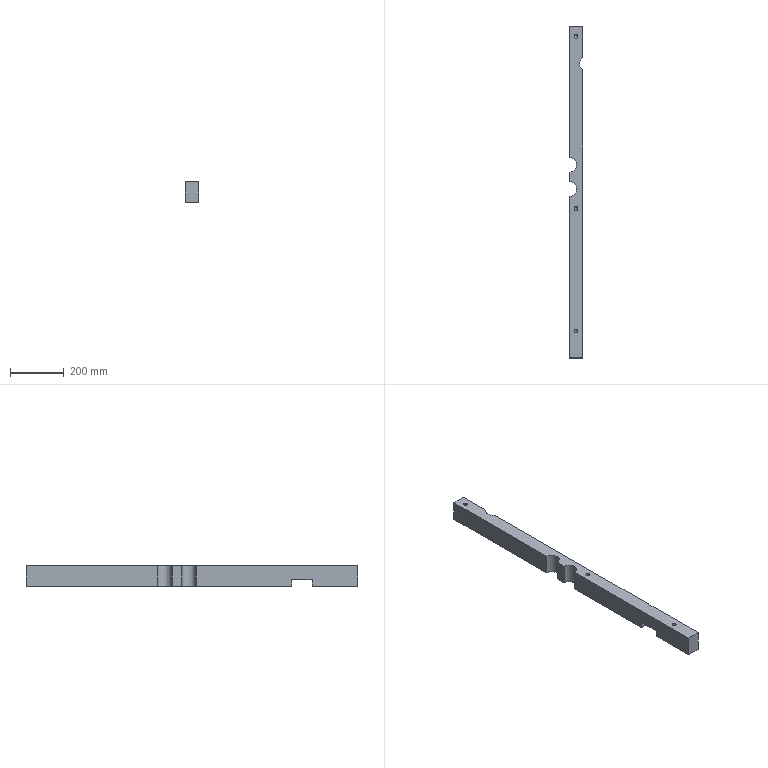Part | NX | features 3 2 | 1 solid | 30 faces | box 50 x 1233 x 75.5 mm | volume 4350206 mm3 | plane 14 | cylinder 10 | cone 6 | commonest cylinder face diameters 14.1 x6 54 x4
STEP:
#1=CARTESIAN_POINT('',(1337.05,-117.5,256.5));
#2=VERTEX_POINT('',#1);
#3=CARTESIAN_POINT('',(1330.,-117.5,256.5));
#4=DIRECTION('',(0.,0.,-1.));
#5=DIRECTION('',(1.,0.,0.));
#6=AXIS2_PLACEMENT_3D('',#3,#4,#5);
#7=CIRCLE('',#6,7.05);
#8=EDGE_CURVE('',#2,#2,#7,.T.);
#9=ORIENTED_EDGE('',*,*,#8,.T.);
#10=EDGE_LOOP('',(#9));
#11=FACE_BOUND('',#10,.T.);
#12=CARTESIAN_POINT('',(1305.,-672.5,256.5));
#13=VERTEX_POINT('',#12);
#14=CARTESIAN_POINT('',(1305.,-72.,256.5));
#15=VERTEX_POINT('',#14);
#16=CARTESIAN_POINT('',(1305.,193.,256.5));
#17=DIRECTION('',(0.,1.,0.));
#18=VECTOR('',#17,1000.);
#19=LINE('',#16,#18);
#20=EDGE_CURVE('',#13,#15,#19,.T.);
#21=ORIENTED_EDGE('',*,*,#20,.F.);
#22=CARTESIAN_POINT('',(1355.,-672.5,256.5));
#23=VERTEX_POINT('',#22);
#24=CARTESIAN_POINT('',(1210.,-672.5,256.5));
#25=DIRECTION('',(-1.,0.,0.));
#26=VECTOR('',#25,1000.);
#27=LINE('',#24,#26);
#28=EDGE_CURVE('',#23,#13,#27,.T.);
#29=ORIENTED_EDGE('',*,*,#28,.F.);
#30=CARTESIAN_POINT('',(1355.,-430.198,256.5));
#31=VERTEX_POINT('',#30);
#32=CARTESIAN_POINT('',(1355.,-526.,256.5));
#33=DIRECTION('',(0.,1.,0.));
#34=VECTOR('',#33,1000.);
#35=LINE('',#32,#34);
#36=EDGE_CURVE('',#23,#31,#35,.T.);
#37=ORIENTED_EDGE('',*,*,#36,.T.);
#38=CARTESIAN_POINT('',(1355.,-409.802,256.5));
#39=VERTEX_POINT('',#38);
#40=CARTESIAN_POINT('',(1380.,-420.,256.5));
#41=DIRECTION('',(0.,0.,1.));
#42=DIRECTION('',(1.,0.,0.));
#43=AXIS2_PLACEMENT_3D('',#40,#41,#42);
#44=CIRCLE('',#43,27.);
#45=EDGE_CURVE('',#39,#31,#44,.T.);
#46=ORIENTED_EDGE('',*,*,#45,.F.);
#47=CARTESIAN_POINT('',(1355.,397.55,256.5));
#48=VERTEX_POINT('',#47);
#49=CARTESIAN_POINT('',(1355.,193.,256.5));
#50=DIRECTION('',(0.,-1.,0.));
#51=VECTOR('',#50,1000.);
#52=LINE('',#49,#51);
#53=EDGE_CURVE('',#48,#39,#52,.T.);
#54=ORIENTED_EDGE('',*,*,#53,.F.);
#55=CARTESIAN_POINT('',(1355.,442.45,256.5));
#56=VERTEX_POINT('',#55);
#57=CARTESIAN_POINT('',(1370.,420.,256.5));
#58=DIRECTION('',(0.,0.,-1.));
#59=DIRECTION('',(1.,0.,0.));
#60=AXIS2_PLACEMENT_3D('',#57,#58,#59);
#61=CIRCLE('',#60,27.);
#62=EDGE_CURVE('',#48,#56,#61,.T.);
#63=ORIENTED_EDGE('',*,*,#62,.T.);
#64=CARTESIAN_POINT('',(1355.,560.5,256.5));
#65=VERTEX_POINT('',#64);
#66=CARTESIAN_POINT('',(1355.,193.,256.5));
#67=DIRECTION('',(0.,-1.,0.));
#68=VECTOR('',#67,1000.);
#69=LINE('',#66,#68);
#70=EDGE_CURVE('',#65,#56,#69,.T.);
#71=ORIENTED_EDGE('',*,*,#70,.F.);
#72=CARTESIAN_POINT('',(1305.,560.5,256.5));
#73=VERTEX_POINT('',#72);
#74=CARTESIAN_POINT('',(3345.,560.5,256.5));
#75=DIRECTION('',(-1.,0.,0.));
#76=VECTOR('',#75,1000.);
#77=LINE('',#74,#76);
#78=EDGE_CURVE('',#65,#73,#77,.T.);
#79=ORIENTED_EDGE('',*,*,#78,.T.);
#80=CARTESIAN_POINT('',(1305.,72.,256.5));
#81=VERTEX_POINT('',#80);
#82=CARTESIAN_POINT('',(1305.,193.,256.5));
#83=DIRECTION('',(0.,1.,0.));
#84=VECTOR('',#83,1000.);
#85=LINE('',#82,#84);
#86=EDGE_CURVE('',#81,#73,#85,.T.);
#87=ORIENTED_EDGE('',*,*,#86,.F.);
#88=CARTESIAN_POINT('',(1305.,18.,256.5));
#89=VERTEX_POINT('',#88);
#90=CARTESIAN_POINT('',(1305.,45.,256.5));
#91=DIRECTION('',(0.,0.,-1.));
#92=DIRECTION('',(1.,0.,0.));
#93=AXIS2_PLACEMENT_3D('',#90,#91,#92);
#94=CIRCLE('',#93,27.);
#95=EDGE_CURVE('',#81,#89,#94,.T.);
#96=ORIENTED_EDGE('',*,*,#95,.T.);
#97=CARTESIAN_POINT('',(1305.,-18.,256.5));
#98=VERTEX_POINT('',#97);
#99=CARTESIAN_POINT('',(1305.,193.,256.5));
#100=DIRECTION('',(0.,1.,0.));
#101=VECTOR('',#100,1000.);
#102=LINE('',#99,#101);
#103=EDGE_CURVE('',#98,#89,#102,.T.);
#104=ORIENTED_EDGE('',*,*,#103,.F.);
#105=CARTESIAN_POINT('',(1305.,-45.,256.5));
#106=DIRECTION('',(0.,0.,1.));
#107=DIRECTION('',(1.,0.,0.));
#108=AXIS2_PLACEMENT_3D('',#105,#106,#107);
#109=CIRCLE('',#108,27.);
#110=EDGE_CURVE('',#15,#98,#109,.T.);
#111=ORIENTED_EDGE('',*,*,#110,.F.);
#112=EDGE_LOOP('',(#21,#29,#37,#46,#54,#63,#71,#79,#87,#96,#104,#111));
#113=FACE_BOUND('',#112,.T.);
#114=CARTESIAN_POINT('',(1337.05,-572.5,256.5));
#115=VERTEX_POINT('',#114);
#116=CARTESIAN_POINT('',(1330.,-572.5,256.5));
#117=DIRECTION('',(0.,0.,-1.));
#118=DIRECTION('',(1.,0.,0.));
#119=AXIS2_PLACEMENT_3D('',#116,#117,#118);
#120=CIRCLE('',#119,7.05);
#121=EDGE_CURVE('',#115,#115,#120,.T.);
#122=ORIENTED_EDGE('',*,*,#121,.T.);
#123=EDGE_LOOP('',(#122));
#124=FACE_BOUND('',#123,.T.);
#125=CARTESIAN_POINT('',(1337.05,522.5,256.5));
#126=VERTEX_POINT('',#125);
#127=CARTESIAN_POINT('',(1330.,522.5,256.5));
#128=DIRECTION('',(0.,0.,-1.));
#129=DIRECTION('',(1.,0.,0.));
#130=AXIS2_PLACEMENT_3D('',#127,#128,#129);
#131=CIRCLE('',#130,7.05);
#132=EDGE_CURVE('',#126,#126,#131,.T.);
#133=ORIENTED_EDGE('',*,*,#132,.T.);
#134=EDGE_LOOP('',(#133));
#135=FACE_BOUND('',#134,.T.);
#136=CARTESIAN_POINT('',(3345.,0.,256.5));
#137=DIRECTION('',(0.,0.,1.));
#138=DIRECTION('',(-1.,0.,0.));
#139=AXIS2_PLACEMENT_3D('',#136,#137,#138);
#140=PLANE('',#139);
#141=ADVANCED_FACE('',(#11,#113,#124,#135),#140,.T.);
#142=CARTESIAN_POINT('',(1337.05,-117.5,181.));
#143=VERTEX_POINT('',#142);
#144=CARTESIAN_POINT('',(1330.,-117.5,181.));
#145=DIRECTION('',(0.,0.,1.));
#146=DIRECTION('',(1.,0.,0.));
#147=AXIS2_PLACEMENT_3D('',#144,#145,#146);
#148=CIRCLE('',#147,7.05);
#149=EDGE_CURVE('',#143,#143,#148,.T.);
#150=ORIENTED_EDGE('',*,*,#149,.T.);
#151=EDGE_LOOP('',(#150));
#152=FACE_BOUND('',#151,.T.);
#153=CARTESIAN_POINT('',(1305.,-426.,181.));
#154=VERTEX_POINT('',#153);
#155=CARTESIAN_POINT('',(1353.675,-426.,181.));
#156=VERTEX_POINT('',#155);
#157=CARTESIAN_POINT('',(2575.,-426.,181.));
#158=DIRECTION('',(1.,0.,0.));
#159=VECTOR('',#158,1000.);
#160=LINE('',#157,#159);
#161=EDGE_CURVE('',#154,#156,#160,.T.);
#162=ORIENTED_EDGE('',*,*,#161,.F.);
#163=CARTESIAN_POINT('',(1305.,-72.,181.));
#164=VERTEX_POINT('',#163);
#165=CARTESIAN_POINT('',(1305.,193.,181.));
#166=DIRECTION('',(0.,-1.,0.));
#167=VECTOR('',#166,1000.);
#168=LINE('',#165,#167);
#169=EDGE_CURVE('',#164,#154,#168,.T.);
#170=ORIENTED_EDGE('',*,*,#169,.F.);
#171=CARTESIAN_POINT('',(1305.,-18.,181.));
#172=VERTEX_POINT('',#171);
#173=CARTESIAN_POINT('',(1305.,-45.,181.));
#174=DIRECTION('',(0.,0.,1.));
#175=DIRECTION('',(-1.,0.,0.));
#176=AXIS2_PLACEMENT_3D('',#173,#174,#175);
#177=CIRCLE('',#176,27.);
#178=EDGE_CURVE('',#164,#172,#177,.T.);
#179=ORIENTED_EDGE('',*,*,#178,.T.);
#180=CARTESIAN_POINT('',(1305.,18.,181.));
#181=VERTEX_POINT('',#180);
#182=CARTESIAN_POINT('',(1305.,193.,181.));
#183=DIRECTION('',(0.,-1.,0.));
#184=VECTOR('',#183,1000.);
#185=LINE('',#182,#184);
#186=EDGE_CURVE('',#181,#172,#185,.T.);
#187=ORIENTED_EDGE('',*,*,#186,.F.);
#188=CARTESIAN_POINT('',(1305.,72.,181.));
#189=VERTEX_POINT('',#188);
#190=CARTESIAN_POINT('',(1305.,45.,181.));
#191=DIRECTION('',(0.,0.,-1.));
#192=DIRECTION('',(-1.,0.,0.));
#193=AXIS2_PLACEMENT_3D('',#190,#191,#192);
#194=CIRCLE('',#193,27.);
#195=EDGE_CURVE('',#189,#181,#194,.T.);
#196=ORIENTED_EDGE('',*,*,#195,.F.);
#197=CARTESIAN_POINT('',(1305.,560.5,181.));
#198=VERTEX_POINT('',#197);
#199=CARTESIAN_POINT('',(1305.,193.,181.));
#200=DIRECTION('',(0.,-1.,0.));
#201=VECTOR('',#200,1000.);
#202=LINE('',#199,#201);
#203=EDGE_CURVE('',#198,#189,#202,.T.);
#204=ORIENTED_EDGE('',*,*,#203,.F.);
#205=CARTESIAN_POINT('',(1355.,560.5,181.));
#206=VERTEX_POINT('',#205);
#207=CARTESIAN_POINT('',(2575.,560.5,181.));
#208=DIRECTION('',(1.,0.,0.));
#209=VECTOR('',#208,1000.);
#210=LINE('',#207,#209);
#211=EDGE_CURVE('',#198,#206,#210,.T.);
#212=ORIENTED_EDGE('',*,*,#211,.T.);
#213=CARTESIAN_POINT('',(1355.,442.45,181.));
#214=VERTEX_POINT('',#213);
#215=CARTESIAN_POINT('',(1355.,193.,181.));
#216=DIRECTION('',(0.,1.,0.));
#217=VECTOR('',#216,1000.);
#218=LINE('',#215,#217);
#219=EDGE_CURVE('',#214,#206,#218,.T.);
#220=ORIENTED_EDGE('',*,*,#219,.F.);
#221=CARTESIAN_POINT('',(1355.,397.55,181.));
#222=VERTEX_POINT('',#221);
#223=CARTESIAN_POINT('',(1370.,420.,181.));
#224=DIRECTION('',(0.,0.,1.));
#225=DIRECTION('',(-1.,0.,0.));
#226=AXIS2_PLACEMENT_3D('',#223,#224,#225);
#227=CIRCLE('',#226,27.);
#228=EDGE_CURVE('',#214,#222,#227,.T.);
#229=ORIENTED_EDGE('',*,*,#228,.T.);
#230=CARTESIAN_POINT('',(1355.,-409.802,181.));
#231=VERTEX_POINT('',#230);
#232=CARTESIAN_POINT('',(1355.,193.,181.));
#233=DIRECTION('',(0.,1.,0.));
#234=VECTOR('',#233,1000.);
#235=LINE('',#232,#234);
#236=EDGE_CURVE('',#231,#222,#235,.T.);
#237=ORIENTED_EDGE('',*,*,#236,.F.);
#238=CARTESIAN_POINT('',(1380.,-420.,181.));
#239=DIRECTION('',(0.,0.,1.));
#240=DIRECTION('',(-1.,0.,0.));
#241=AXIS2_PLACEMENT_3D('',#238,#239,#240);
#242=CIRCLE('',#241,27.);
#243=EDGE_CURVE('',#231,#156,#242,.T.);
#244=ORIENTED_EDGE('',*,*,#243,.T.);
#245=EDGE_LOOP('',(#162,#170,#179,#187,#196,#204,#212,#220,#229,#237,#244));
#246=FACE_BOUND('',#245,.T.);
#247=CARTESIAN_POINT('',(1337.05,522.5,181.));
#248=VERTEX_POINT('',#247);
#249=CARTESIAN_POINT('',(1330.,522.5,181.));
#250=DIRECTION('',(0.,0.,1.));
#251=DIRECTION('',(1.,0.,0.));
#252=AXIS2_PLACEMENT_3D('',#249,#250,#251);
#253=CIRCLE('',#252,7.05);
#254=EDGE_CURVE('',#248,#248,#253,.T.);
#255=ORIENTED_EDGE('',*,*,#254,.T.);
#256=EDGE_LOOP('',(#255));
#257=FACE_BOUND('',#256,.T.);
#258=CARTESIAN_POINT('',(2575.,193.,181.));
#259=DIRECTION('',(0.,0.,-1.));
#260=DIRECTION('',(-1.,0.,0.));
#261=AXIS2_PLACEMENT_3D('',#258,#259,#260);
#262=PLANE('',#261);
#263=ADVANCED_FACE('',(#152,#246,#257),#262,.T.);
#264=CARTESIAN_POINT('',(1355.,-502.,181.));
#265=VERTEX_POINT('',#264);
#266=CARTESIAN_POINT('',(1305.,-502.,181.));
#267=VERTEX_POINT('',#266);
#268=CARTESIAN_POINT('',(2575.,-502.,181.));
#269=DIRECTION('',(-1.,0.,0.));
#270=VECTOR('',#269,1000.);
#271=LINE('',#268,#270);
#272=EDGE_CURVE('',#265,#267,#271,.T.);
#273=ORIENTED_EDGE('',*,*,#272,.F.);
#274=CARTESIAN_POINT('',(1355.,-672.5,181.));
#275=VERTEX_POINT('',#274);
#276=CARTESIAN_POINT('',(1355.,-526.,181.));
#277=DIRECTION('',(0.,1.,0.));
#278=VECTOR('',#277,1000.);
#279=LINE('',#276,#278);
#280=EDGE_CURVE('',#275,#265,#279,.T.);
#281=ORIENTED_EDGE('',*,*,#280,.F.);
#282=CARTESIAN_POINT('',(1305.,-672.5,181.));
#283=VERTEX_POINT('',#282);
#284=CARTESIAN_POINT('',(2575.,-672.5,181.));
#285=DIRECTION('',(-1.,0.,0.));
#286=VECTOR('',#285,1000.);
#287=LINE('',#284,#286);
#288=EDGE_CURVE('',#275,#283,#287,.T.);
#289=ORIENTED_EDGE('',*,*,#288,.T.);
#290=CARTESIAN_POINT('',(1305.,193.,181.));
#291=DIRECTION('',(0.,-1.,0.));
#292=VECTOR('',#291,1000.);
#293=LINE('',#290,#292);
#294=EDGE_CURVE('',#267,#283,#293,.T.);
#295=ORIENTED_EDGE('',*,*,#294,.F.);
#296=EDGE_LOOP('',(#273,#281,#289,#295));
#297=FACE_BOUND('',#296,.T.);
#298=CARTESIAN_POINT('',(1337.05,-572.5,181.));
#299=VERTEX_POINT('',#298);
#300=CARTESIAN_POINT('',(1330.,-572.5,181.));
#301=DIRECTION('',(0.,0.,1.));
#302=DIRECTION('',(1.,0.,0.));
#303=AXIS2_PLACEMENT_3D('',#300,#301,#302);
#304=CIRCLE('',#303,7.05);
#305=EDGE_CURVE('',#299,#299,#304,.T.);
#306=ORIENTED_EDGE('',*,*,#305,.T.);
#307=EDGE_LOOP('',(#306));
#308=FACE_BOUND('',#307,.T.);
#309=CARTESIAN_POINT('',(2575.,193.,181.));
#310=DIRECTION('',(0.,0.,-1.));
#311=DIRECTION('',(-1.,0.,0.));
#312=AXIS2_PLACEMENT_3D('',#309,#310,#311);
#313=PLANE('',#312);
#314=ADVANCED_FACE('',(#297,#308),#313,.T.);
#315=CARTESIAN_POINT('',(1355.,-430.198,205.));
#316=VERTEX_POINT('',#315);
#317=CARTESIAN_POINT('',(1355.,-502.,205.));
#318=VERTEX_POINT('',#317);
#319=CARTESIAN_POINT('',(1355.,193.,205.));
#320=DIRECTION('',(0.,-1.,0.));
#321=VECTOR('',#320,1000.);
#322=LINE('',#319,#321);
#323=EDGE_CURVE('',#316,#318,#322,.T.);
#324=ORIENTED_EDGE('',*,*,#323,.F.);
#325=CARTESIAN_POINT('',(1355.,-430.198,-181.));
#326=DIRECTION('',(0.,0.,-1.));
#327=VECTOR('',#326,1000.);
#328=LINE('',#325,#327);
#329=EDGE_CURVE('',#31,#316,#328,.T.);
#330=ORIENTED_EDGE('',*,*,#329,.F.);
#331=ORIENTED_EDGE('',*,*,#36,.F.);
#332=CARTESIAN_POINT('',(1355.,-672.5,-1.5));
#333=DIRECTION('',(0.,0.,1.));
#334=VECTOR('',#333,1000.);
#335=LINE('',#332,#334);
#336=EDGE_CURVE('',#275,#23,#335,.T.);
#337=ORIENTED_EDGE('',*,*,#336,.F.);
#338=ORIENTED_EDGE('',*,*,#280,.T.);
#339=CARTESIAN_POINT('',(1355.,-502.,25.));
#340=DIRECTION('',(0.,0.,1.));
#341=VECTOR('',#340,1000.);
#342=LINE('',#339,#341);
#343=EDGE_CURVE('',#265,#318,#342,.T.);
#344=ORIENTED_EDGE('',*,*,#343,.T.);
#345=EDGE_LOOP('',(#324,#330,#331,#337,#338,#344));
#346=FACE_BOUND('',#345,.T.);
#347=CARTESIAN_POINT('',(1355.,193.,-1.5));
#348=DIRECTION('',(1.,0.,0.));
#349=DIRECTION('',(0.,0.,1.));
#350=AXIS2_PLACEMENT_3D('',#347,#348,#349);
#351=PLANE('',#350);
#352=ADVANCED_FACE('',(#346),#351,.T.);
#353=CARTESIAN_POINT('',(1355.,-409.802,-181.));
#354=DIRECTION('',(0.,0.,1.));
#355=VECTOR('',#354,1000.);
#356=LINE('',#353,#355);
#357=EDGE_CURVE('',#231,#39,#356,.T.);
#358=ORIENTED_EDGE('',*,*,#357,.F.);
#359=ORIENTED_EDGE('',*,*,#236,.T.);
#360=CARTESIAN_POINT('',(1355.,397.55,-181.));
#361=DIRECTION('',(0.,0.,-1.));
#362=VECTOR('',#361,1000.);
#363=LINE('',#360,#362);
#364=EDGE_CURVE('',#48,#222,#363,.T.);
#365=ORIENTED_EDGE('',*,*,#364,.F.);
#366=ORIENTED_EDGE('',*,*,#53,.T.);
#367=EDGE_LOOP('',(#358,#359,#365,#366));
#368=FACE_BOUND('',#367,.T.);
#369=CARTESIAN_POINT('',(1355.,193.,-1.5));
#370=DIRECTION('',(1.,0.,0.));
#371=DIRECTION('',(0.,0.,1.));
#372=AXIS2_PLACEMENT_3D('',#369,#370,#371);
#373=PLANE('',#372);
#374=ADVANCED_FACE('',(#368),#373,.T.);
#375=ORIENTED_EDGE('',*,*,#70,.T.);
#376=CARTESIAN_POINT('',(1355.,442.45,-181.));
#377=DIRECTION('',(0.,0.,1.));
#378=VECTOR('',#377,1000.);
#379=LINE('',#376,#378);
#380=EDGE_CURVE('',#214,#56,#379,.T.);
#381=ORIENTED_EDGE('',*,*,#380,.F.);
#382=ORIENTED_EDGE('',*,*,#219,.T.);
#383=CARTESIAN_POINT('',(1355.,560.5,-1.5));
#384=DIRECTION('',(0.,0.,1.));
#385=VECTOR('',#384,1000.);
#386=LINE('',#383,#385);
#387=EDGE_CURVE('',#206,#65,#386,.T.);
#388=ORIENTED_EDGE('',*,*,#387,.T.);
#389=EDGE_LOOP('',(#375,#381,#382,#388));
#390=FACE_BOUND('',#389,.T.);
#391=CARTESIAN_POINT('',(1355.,193.,-1.5));
#392=DIRECTION('',(1.,0.,0.));
#393=DIRECTION('',(0.,0.,1.));
#394=AXIS2_PLACEMENT_3D('',#391,#392,#393);
#395=PLANE('',#394);
#396=ADVANCED_FACE('',(#390),#395,.T.);
#397=ORIENTED_EDGE('',*,*,#103,.T.);
#398=CARTESIAN_POINT('',(1305.,18.,-181.));
#399=DIRECTION('',(0.,0.,1.));
#400=VECTOR('',#399,1000.);
#401=LINE('',#398,#400);
#402=EDGE_CURVE('',#181,#89,#401,.T.);
#403=ORIENTED_EDGE('',*,*,#402,.F.);
#404=ORIENTED_EDGE('',*,*,#186,.T.);
#405=CARTESIAN_POINT('',(1305.,-18.,181.));
#406=DIRECTION('',(0.,0.,1.));
#407=VECTOR('',#406,1000.);
#408=LINE('',#405,#407);
#409=EDGE_CURVE('',#172,#98,#408,.T.);
#410=ORIENTED_EDGE('',*,*,#409,.T.);
#411=EDGE_LOOP('',(#397,#403,#404,#410));
#412=FACE_BOUND('',#411,.T.);
#413=CARTESIAN_POINT('',(1305.,193.,-1.5));
#414=DIRECTION('',(-1.,0.,0.));
#415=DIRECTION('',(0.,0.,-1.));
#416=AXIS2_PLACEMENT_3D('',#413,#414,#415);
#417=PLANE('',#416);
#418=ADVANCED_FACE('',(#412),#417,.T.);
#419=ORIENTED_EDGE('',*,*,#203,.T.);
#420=CARTESIAN_POINT('',(1305.,72.,256.5));
#421=DIRECTION('',(0.,0.,-1.));
#422=VECTOR('',#421,1000.);
#423=LINE('',#420,#422);
#424=EDGE_CURVE('',#81,#189,#423,.T.);
#425=ORIENTED_EDGE('',*,*,#424,.F.);
#426=ORIENTED_EDGE('',*,*,#86,.T.);
#427=CARTESIAN_POINT('',(1305.,560.5,-1.5));
#428=DIRECTION('',(0.,0.,-1.));
#429=VECTOR('',#428,1000.);
#430=LINE('',#427,#429);
#431=EDGE_CURVE('',#73,#198,#430,.T.);
#432=ORIENTED_EDGE('',*,*,#431,.T.);
#433=EDGE_LOOP('',(#419,#425,#426,#432));
#434=FACE_BOUND('',#433,.T.);
#435=CARTESIAN_POINT('',(1305.,193.,-1.5));
#436=DIRECTION('',(-1.,0.,0.));
#437=DIRECTION('',(0.,0.,-1.));
#438=AXIS2_PLACEMENT_3D('',#435,#436,#437);
#439=PLANE('',#438);
#440=ADVANCED_FACE('',(#434),#439,.T.);
#441=CARTESIAN_POINT('',(1305.,-502.,205.));
#442=VERTEX_POINT('',#441);
#443=CARTESIAN_POINT('',(1305.,-502.,-1.5));
#444=DIRECTION('',(0.,0.,1.));
#445=VECTOR('',#444,1000.);
#446=LINE('',#443,#445);
#447=EDGE_CURVE('',#267,#442,#446,.T.);
#448=ORIENTED_EDGE('',*,*,#447,.F.);
#449=ORIENTED_EDGE('',*,*,#294,.T.);
#450=CARTESIAN_POINT('',(1305.,-672.5,-1.5));
#451=DIRECTION('',(0.,0.,1.));
#452=VECTOR('',#451,1000.);
#453=LINE('',#450,#452);
#454=EDGE_CURVE('',#283,#13,#453,.T.);
#455=ORIENTED_EDGE('',*,*,#454,.T.);
#456=ORIENTED_EDGE('',*,*,#20,.T.);
#457=CARTESIAN_POINT('',(1305.,-72.,-181.));
#458=DIRECTION('',(0.,0.,-1.));
#459=VECTOR('',#458,1000.);
#460=LINE('',#457,#459);
#461=EDGE_CURVE('',#15,#164,#460,.T.);
#462=ORIENTED_EDGE('',*,*,#461,.T.);
#463=ORIENTED_EDGE('',*,*,#169,.T.);
#464=CARTESIAN_POINT('',(1305.,-426.,205.));
#465=VERTEX_POINT('',#464);
#466=CARTESIAN_POINT('',(1305.,-426.,-1.5));
#467=DIRECTION('',(0.,0.,-1.));
#468=VECTOR('',#467,1000.);
#469=LINE('',#466,#468);
#470=EDGE_CURVE('',#465,#154,#469,.T.);
#471=ORIENTED_EDGE('',*,*,#470,.F.);
#472=CARTESIAN_POINT('',(1305.,193.,205.));
#473=DIRECTION('',(0.,1.,0.));
#474=VECTOR('',#473,1000.);
#475=LINE('',#472,#474);
#476=EDGE_CURVE('',#442,#465,#475,.T.);
#477=ORIENTED_EDGE('',*,*,#476,.F.);
#478=EDGE_LOOP('',(#448,#449,#455,#456,#462,#463,#471,#477));
#479=FACE_BOUND('',#478,.T.);
#480=CARTESIAN_POINT('',(1305.,193.,-1.5));
#481=DIRECTION('',(-1.,0.,0.));
#482=DIRECTION('',(0.,0.,-1.));
#483=AXIS2_PLACEMENT_3D('',#480,#481,#482);
#484=PLANE('',#483);
#485=ADVANCED_FACE('',(#479),#484,.T.);
#486=ORIENTED_EDGE('',*,*,#78,.F.);
#487=ORIENTED_EDGE('',*,*,#387,.F.);
#488=ORIENTED_EDGE('',*,*,#211,.F.);
#489=ORIENTED_EDGE('',*,*,#431,.F.);
#490=EDGE_LOOP('',(#486,#487,#488,#489));
#491=FACE_BOUND('',#490,.T.);
#492=CARTESIAN_POINT('',(1275.,560.5,179.));
#493=DIRECTION('',(0.,1.,0.));
#494=DIRECTION('',(0.,0.,-1.));
#495=AXIS2_PLACEMENT_3D('',#492,#493,#494);
#496=PLANE('',#495);
#497=ADVANCED_FACE('',(#491),#496,.T.);
#498=ORIENTED_EDGE('',*,*,#110,.T.);
#499=ORIENTED_EDGE('',*,*,#409,.F.);
#500=ORIENTED_EDGE('',*,*,#178,.F.);
#501=ORIENTED_EDGE('',*,*,#461,.F.);
#502=EDGE_LOOP('',(#498,#499,#500,#501));
#503=FACE_BOUND('',#502,.T.);
#504=CARTESIAN_POINT('',(1305.,-45.,-181.));
#505=DIRECTION('',(0.,0.,1.));
#506=DIRECTION('',(-1.,0.,0.));
#507=AXIS2_PLACEMENT_3D('',#504,#505,#506);
#508=CYLINDRICAL_SURFACE('',#507,27.);
#509=ADVANCED_FACE('',(#503),#508,.F.);
#510=ORIENTED_EDGE('',*,*,#95,.F.);
#511=ORIENTED_EDGE('',*,*,#424,.T.);
#512=ORIENTED_EDGE('',*,*,#195,.T.);
#513=ORIENTED_EDGE('',*,*,#402,.T.);
#514=EDGE_LOOP('',(#510,#511,#512,#513));
#515=FACE_BOUND('',#514,.T.);
#516=CARTESIAN_POINT('',(1305.,45.,-181.));
#517=DIRECTION('',(0.,0.,1.));
#518=DIRECTION('',(-1.,0.,0.));
#519=AXIS2_PLACEMENT_3D('',#516,#517,#518);
#520=CYLINDRICAL_SURFACE('',#519,27.);
#521=ADVANCED_FACE('',(#515),#520,.F.);
#522=ORIENTED_EDGE('',*,*,#380,.T.);
#523=ORIENTED_EDGE('',*,*,#62,.F.);
#524=ORIENTED_EDGE('',*,*,#364,.T.);
#525=ORIENTED_EDGE('',*,*,#228,.F.);
#526=EDGE_LOOP('',(#522,#523,#524,#525));
#527=FACE_BOUND('',#526,.T.);
#528=CARTESIAN_POINT('',(1370.,420.,-181.));
#529=DIRECTION('',(0.,0.,1.));
#530=DIRECTION('',(-1.,0.,0.));
#531=AXIS2_PLACEMENT_3D('',#528,#529,#530);
#532=CYLINDRICAL_SURFACE('',#531,27.);
#533=ADVANCED_FACE('',(#527),#532,.F.);
#534=ORIENTED_EDGE('',*,*,#329,.T.);
#535=CARTESIAN_POINT('',(1353.675,-426.,205.));
#536=VERTEX_POINT('',#535);
#537=CARTESIAN_POINT('',(1380.,-420.,205.));
#538=DIRECTION('',(0.,0.,-1.));
#539=DIRECTION('',(1.,0.,0.));
#540=AXIS2_PLACEMENT_3D('',#537,#538,#539);
#541=CIRCLE('',#540,27.);
#542=EDGE_CURVE('',#316,#536,#541,.T.);
#543=ORIENTED_EDGE('',*,*,#542,.T.);
#544=CARTESIAN_POINT('',(1353.675,-426.,-181.));
#545=DIRECTION('',(0.,0.,-1.));
#546=VECTOR('',#545,1000.);
#547=LINE('',#544,#546);
#548=EDGE_CURVE('',#536,#156,#547,.T.);
#549=ORIENTED_EDGE('',*,*,#548,.T.);
#550=ORIENTED_EDGE('',*,*,#243,.F.);
#551=ORIENTED_EDGE('',*,*,#357,.T.);
#552=ORIENTED_EDGE('',*,*,#45,.T.);
#553=EDGE_LOOP('',(#534,#543,#549,#550,#551,#552));
#554=FACE_BOUND('',#553,.T.);
#555=CARTESIAN_POINT('',(1380.,-420.,-181.));
#556=DIRECTION('',(0.,0.,1.));
#557=DIRECTION('',(-1.,0.,0.));
#558=AXIS2_PLACEMENT_3D('',#555,#556,#557);
#559=CYLINDRICAL_SURFACE('',#558,27.);
#560=ADVANCED_FACE('',(#554),#559,.F.);
#561=ORIENTED_EDGE('',*,*,#288,.F.);
#562=ORIENTED_EDGE('',*,*,#336,.T.);
#563=ORIENTED_EDGE('',*,*,#28,.T.);
#564=ORIENTED_EDGE('',*,*,#454,.F.);
#565=EDGE_LOOP('',(#561,#562,#563,#564));
#566=FACE_BOUND('',#565,.T.);
#567=CARTESIAN_POINT('',(282.5,-672.5,-103.));
#568=DIRECTION('',(0.,1.,0.));
#569=DIRECTION('',(1.,0.,0.));
#570=AXIS2_PLACEMENT_3D('',#567,#568,#569);
#571=PLANE('',#570);
#572=ADVANCED_FACE('',(#566),#571,.F.);
#573=ORIENTED_EDGE('',*,*,#476,.T.);
#574=CARTESIAN_POINT('',(1262.5,-426.,205.));
#575=DIRECTION('',(-1.,0.,0.));
#576=VECTOR('',#575,1000.);
#577=LINE('',#574,#576);
#578=EDGE_CURVE('',#536,#465,#577,.T.);
#579=ORIENTED_EDGE('',*,*,#578,.F.);
#580=ORIENTED_EDGE('',*,*,#542,.F.);
#581=ORIENTED_EDGE('',*,*,#323,.T.);
#582=CARTESIAN_POINT('',(1262.5,-502.,205.));
#583=DIRECTION('',(1.,0.,0.));
#584=VECTOR('',#583,1000.);
#585=LINE('',#582,#584);
#586=EDGE_CURVE('',#442,#318,#585,.T.);
#587=ORIENTED_EDGE('',*,*,#586,.F.);
#588=EDGE_LOOP('',(#573,#579,#580,#581,#587));
#589=FACE_BOUND('',#588,.T.);
#590=CARTESIAN_POINT('',(1262.5,-464.,205.));
#591=DIRECTION('',(0.,0.,1.));
#592=DIRECTION('',(-1.,0.,0.));
#593=AXIS2_PLACEMENT_3D('',#590,#591,#592);
#594=PLANE('',#593);
#595=ADVANCED_FACE('',(#589),#594,.F.);
#596=ORIENTED_EDGE('',*,*,#272,.T.);
#597=ORIENTED_EDGE('',*,*,#447,.T.);
#598=ORIENTED_EDGE('',*,*,#586,.T.);
#599=ORIENTED_EDGE('',*,*,#343,.F.);
#600=EDGE_LOOP('',(#596,#597,#598,#599));
#601=FACE_BOUND('',#600,.T.);
#602=CARTESIAN_POINT('',(1262.5,-502.,25.));
#603=DIRECTION('',(0.,-1.,0.));
#604=DIRECTION('',(0.,0.,1.));
#605=AXIS2_PLACEMENT_3D('',#602,#603,#604);
#606=PLANE('',#605);
#607=ADVANCED_FACE('',(#601),#606,.F.);
#608=ORIENTED_EDGE('',*,*,#470,.T.);
#609=ORIENTED_EDGE('',*,*,#161,.T.);
#610=ORIENTED_EDGE('',*,*,#548,.F.);
#611=ORIENTED_EDGE('',*,*,#578,.T.);
#612=EDGE_LOOP('',(#608,#609,#610,#611));
#613=FACE_BOUND('',#612,.T.);
#614=CARTESIAN_POINT('',(1262.5,-426.,25.));
#615=DIRECTION('',(0.,1.,0.));
#616=DIRECTION('',(0.,0.,-1.));
#617=AXIS2_PLACEMENT_3D('',#614,#615,#616);
#618=PLANE('',#617);
#619=ADVANCED_FACE('',(#613),#618,.F.);
#620=CARTESIAN_POINT('',(1337.05,-572.5,188.95));
#621=VERTEX_POINT('',#620);
#622=CARTESIAN_POINT('',(1330.,-572.5,188.95));
#623=DIRECTION('',(0.,0.,1.));
#624=DIRECTION('',(1.,0.,0.));
#625=AXIS2_PLACEMENT_3D('',#622,#623,#624);
#626=CIRCLE('',#625,7.05);
#627=EDGE_CURVE('',#621,#621,#626,.T.);
#628=ORIENTED_EDGE('',*,*,#627,.T.);
#629=EDGE_LOOP('',(#628));
#630=FACE_BOUND('',#629,.T.);
#631=ORIENTED_EDGE('',*,*,#305,.F.);
#632=EDGE_LOOP('',(#631));
#633=FACE_BOUND('',#632,.T.);
#634=CARTESIAN_POINT('',(1330.,-572.5,181.));
#635=DIRECTION('',(0.,0.,1.));
#636=DIRECTION('',(-1.,0.,0.));
#637=AXIS2_PLACEMENT_3D('',#634,#635,#636);
#638=CYLINDRICAL_SURFACE('',#637,7.05);
#639=ADVANCED_FACE('',(#630,#633),#638,.F.);
#640=CARTESIAN_POINT('',(1330.,-572.5,196.));
#641=VERTEX_POINT('',#640);
#642=VERTEX_LOOP('',#641);
#643=FACE_BOUND('',#642,.T.);
#644=ORIENTED_EDGE('',*,*,#627,.F.);
#645=EDGE_LOOP('',(#644));
#646=FACE_BOUND('',#645,.T.);
#647=CARTESIAN_POINT('',(1330.,-572.5,188.95));
#648=DIRECTION('',(0.,0.,-1.));
#649=DIRECTION('',(1.,0.,0.));
#650=AXIS2_PLACEMENT_3D('',#647,#648,#649);
#651=CONICAL_SURFACE('',#650,7.05,0.7854);
#652=ADVANCED_FACE('',(#643,#646),#651,.F.);
#653=CARTESIAN_POINT('',(1337.05,-117.5,188.95));
#654=VERTEX_POINT('',#653);
#655=CARTESIAN_POINT('',(1330.,-117.5,188.95));
#656=DIRECTION('',(0.,0.,1.));
#657=DIRECTION('',(1.,0.,0.));
#658=AXIS2_PLACEMENT_3D('',#655,#656,#657);
#659=CIRCLE('',#658,7.05);
#660=EDGE_CURVE('',#654,#654,#659,.T.);
#661=ORIENTED_EDGE('',*,*,#660,.T.);
#662=EDGE_LOOP('',(#661));
#663=FACE_BOUND('',#662,.T.);
#664=ORIENTED_EDGE('',*,*,#149,.F.);
#665=EDGE_LOOP('',(#664));
#666=FACE_BOUND('',#665,.T.);
#667=CARTESIAN_POINT('',(1330.,-117.5,181.));
#668=DIRECTION('',(0.,0.,1.));
#669=DIRECTION('',(-1.,0.,0.));
#670=AXIS2_PLACEMENT_3D('',#667,#668,#669);
#671=CYLINDRICAL_SURFACE('',#670,7.05);
#672=ADVANCED_FACE('',(#663,#666),#671,.F.);
#673=CARTESIAN_POINT('',(1330.,-117.5,196.));
#674=VERTEX_POINT('',#673);
#675=VERTEX_LOOP('',#674);
#676=FACE_BOUND('',#675,.T.);
#677=ORIENTED_EDGE('',*,*,#660,.F.);
#678=EDGE_LOOP('',(#677));
#679=FACE_BOUND('',#678,.T.);
#680=CARTESIAN_POINT('',(1330.,-117.5,188.95));
#681=DIRECTION('',(0.,0.,-1.));
#682=DIRECTION('',(1.,0.,0.));
#683=AXIS2_PLACEMENT_3D('',#680,#681,#682);
#684=CONICAL_SURFACE('',#683,7.05,0.7854);
#685=ADVANCED_FACE('',(#676,#679),#684,.F.);
#686=CARTESIAN_POINT('',(1337.05,522.5,188.95));
#687=VERTEX_POINT('',#686);
#688=CARTESIAN_POINT('',(1330.,522.5,188.95));
#689=DIRECTION('',(0.,0.,1.));
#690=DIRECTION('',(1.,0.,0.));
#691=AXIS2_PLACEMENT_3D('',#688,#689,#690);
#692=CIRCLE('',#691,7.05);
#693=EDGE_CURVE('',#687,#687,#692,.T.);
#694=ORIENTED_EDGE('',*,*,#693,.T.);
#695=EDGE_LOOP('',(#694));
#696=FACE_BOUND('',#695,.T.);
#697=ORIENTED_EDGE('',*,*,#254,.F.);
#698=EDGE_LOOP('',(#697));
#699=FACE_BOUND('',#698,.T.);
#700=CARTESIAN_POINT('',(1330.,522.5,181.));
#701=DIRECTION('',(0.,0.,1.));
#702=DIRECTION('',(-1.,0.,0.));
#703=AXIS2_PLACEMENT_3D('',#700,#701,#702);
#704=CYLINDRICAL_SURFACE('',#703,7.05);
#705=ADVANCED_FACE('',(#696,#699),#704,.F.);
#706=CARTESIAN_POINT('',(1330.,522.5,196.));
#707=VERTEX_POINT('',#706);
#708=VERTEX_LOOP('',#707);
#709=FACE_BOUND('',#708,.T.);
#710=ORIENTED_EDGE('',*,*,#693,.F.);
#711=EDGE_LOOP('',(#710));
#712=FACE_BOUND('',#711,.T.);
#713=CARTESIAN_POINT('',(1330.,522.5,188.95));
#714=DIRECTION('',(0.,0.,-1.));
#715=DIRECTION('',(1.,0.,0.));
#716=AXIS2_PLACEMENT_3D('',#713,#714,#715);
#717=CONICAL_SURFACE('',#716,7.05,0.7854);
#718=ADVANCED_FACE('',(#709,#712),#717,.F.);
#719=CARTESIAN_POINT('',(1322.95,-572.5,248.55));
#720=VERTEX_POINT('',#719);
#721=CARTESIAN_POINT('',(1330.,-572.5,248.55));
#722=DIRECTION('',(0.,0.,-1.));
#723=DIRECTION('',(-1.,0.,0.));
#724=AXIS2_PLACEMENT_3D('',#721,#722,#723);
#725=CIRCLE('',#724,7.05);
#726=EDGE_CURVE('',#720,#720,#725,.T.);
#727=ORIENTED_EDGE('',*,*,#726,.T.);
#728=EDGE_LOOP('',(#727));
#729=FACE_BOUND('',#728,.T.);
#730=ORIENTED_EDGE('',*,*,#121,.F.);
#731=EDGE_LOOP('',(#730));
#732=FACE_BOUND('',#731,.T.);
#733=CARTESIAN_POINT('',(1330.,-572.5,256.5));
#734=DIRECTION('',(0.,0.,-1.));
#735=DIRECTION('',(-1.,0.,0.));
#736=AXIS2_PLACEMENT_3D('',#733,#734,#735);
#737=CYLINDRICAL_SURFACE('',#736,7.05);
#738=ADVANCED_FACE('',(#729,#732),#737,.F.);
#739=CARTESIAN_POINT('',(1330.,-572.5,241.5));
#740=VERTEX_POINT('',#739);
#741=VERTEX_LOOP('',#740);
#742=FACE_BOUND('',#741,.T.);
#743=ORIENTED_EDGE('',*,*,#726,.F.);
#744=EDGE_LOOP('',(#743));
#745=FACE_BOUND('',#744,.T.);
#746=CARTESIAN_POINT('',(1330.,-572.5,248.55));
#747=DIRECTION('',(0.,0.,1.));
#748=DIRECTION('',(-1.,0.,0.));
#749=AXIS2_PLACEMENT_3D('',#746,#747,#748);
#750=CONICAL_SURFACE('',#749,7.05,0.7854);
#751=ADVANCED_FACE('',(#742,#745),#750,.F.);
#752=CARTESIAN_POINT('',(1322.95,-117.5,248.55));
#753=VERTEX_POINT('',#752);
#754=CARTESIAN_POINT('',(1330.,-117.5,248.55));
#755=DIRECTION('',(0.,0.,-1.));
#756=DIRECTION('',(-1.,0.,0.));
#757=AXIS2_PLACEMENT_3D('',#754,#755,#756);
#758=CIRCLE('',#757,7.05);
#759=EDGE_CURVE('',#753,#753,#758,.T.);
#760=ORIENTED_EDGE('',*,*,#759,.T.);
#761=EDGE_LOOP('',(#760));
#762=FACE_BOUND('',#761,.T.);
#763=ORIENTED_EDGE('',*,*,#8,.F.);
#764=EDGE_LOOP('',(#763));
#765=FACE_BOUND('',#764,.T.);
#766=CARTESIAN_POINT('',(1330.,-117.5,256.5));
#767=DIRECTION('',(0.,0.,-1.));
#768=DIRECTION('',(-1.,0.,0.));
#769=AXIS2_PLACEMENT_3D('',#766,#767,#768);
#770=CYLINDRICAL_SURFACE('',#769,7.05);
#771=ADVANCED_FACE('',(#762,#765),#770,.F.);
#772=CARTESIAN_POINT('',(1330.,-117.5,241.5));
#773=VERTEX_POINT('',#772);
#774=VERTEX_LOOP('',#773);
#775=FACE_BOUND('',#774,.T.);
#776=ORIENTED_EDGE('',*,*,#759,.F.);
#777=EDGE_LOOP('',(#776));
#778=FACE_BOUND('',#777,.T.);
#779=CARTESIAN_POINT('',(1330.,-117.5,248.55));
#780=DIRECTION('',(0.,0.,1.));
#781=DIRECTION('',(-1.,0.,0.));
#782=AXIS2_PLACEMENT_3D('',#779,#780,#781);
#783=CONICAL_SURFACE('',#782,7.05,0.7854);
#784=ADVANCED_FACE('',(#775,#778),#783,.F.);
#785=CARTESIAN_POINT('',(1322.95,522.5,248.55));
#786=VERTEX_POINT('',#785);
#787=CARTESIAN_POINT('',(1330.,522.5,248.55));
#788=DIRECTION('',(0.,0.,-1.));
#789=DIRECTION('',(-1.,0.,0.));
#790=AXIS2_PLACEMENT_3D('',#787,#788,#789);
#791=CIRCLE('',#790,7.05);
#792=EDGE_CURVE('',#786,#786,#791,.T.);
#793=ORIENTED_EDGE('',*,*,#792,.T.);
#794=EDGE_LOOP('',(#793));
#795=FACE_BOUND('',#794,.T.);
#796=ORIENTED_EDGE('',*,*,#132,.F.);
#797=EDGE_LOOP('',(#796));
#798=FACE_BOUND('',#797,.T.);
#799=CARTESIAN_POINT('',(1330.,522.5,256.5));
#800=DIRECTION('',(0.,0.,-1.));
#801=DIRECTION('',(-1.,0.,0.));
#802=AXIS2_PLACEMENT_3D('',#799,#800,#801);
#803=CYLINDRICAL_SURFACE('',#802,7.05);
#804=ADVANCED_FACE('',(#795,#798),#803,.F.);
#805=CARTESIAN_POINT('',(1330.,522.5,241.5));
#806=VERTEX_POINT('',#805);
#807=VERTEX_LOOP('',#806);
#808=FACE_BOUND('',#807,.T.);
#809=ORIENTED_EDGE('',*,*,#792,.F.);
#810=EDGE_LOOP('',(#809));
#811=FACE_BOUND('',#810,.T.);
#812=CARTESIAN_POINT('',(1330.,522.5,248.55));
#813=DIRECTION('',(0.,0.,1.));
#814=DIRECTION('',(-1.,0.,0.));
#815=AXIS2_PLACEMENT_3D('',#812,#813,#814);
#816=CONICAL_SURFACE('',#815,7.05,0.7854);
#817=ADVANCED_FACE('',(#808,#811),#816,.F.);
#818=CLOSED_SHELL('',(#141,#263,#314,#352,#374,#396,#418,#440,#485,#497,#509,#521,#533,#560,#572,#595,#607,#619,#639,#652,#672,#685,#705,#718,#738,#751,#771,#784,#804,#817));
#819=MANIFOLD_SOLID_BREP('',#818);
#820=(LENGTH_UNIT()NAMED_UNIT(*)SI_UNIT(.MILLI.,.METRE.));
#821=UNCERTAINTY_MEASURE_WITH_UNIT(LENGTH_MEASURE(0.00001),#820,'','');
#822=(NAMED_UNIT(*)PLANE_ANGLE_UNIT()SI_UNIT($,.RADIAN.));
#823=(NAMED_UNIT(*)SI_UNIT($,.STERADIAN.)SOLID_ANGLE_UNIT());
#824=(GEOMETRIC_REPRESENTATION_CONTEXT(3)GLOBAL_UNCERTAINTY_ASSIGNED_CONTEXT((#821))GLOBAL_UNIT_ASSIGNED_CONTEXT((#820,#822,#823))REPRESENTATION_CONTEXT('',''));
#825=ADVANCED_BREP_SHAPE_REPRESENTATION('',(#819),#824);